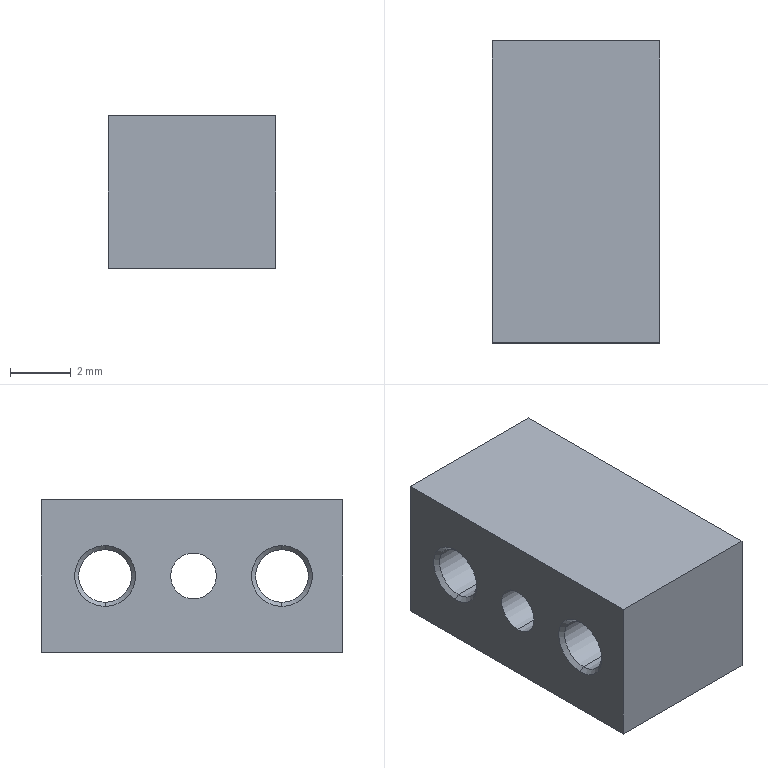Part | STEP file | 1 solid | 20 faces | box 5.5 x 9.9 x 5 mm | volume 236.494 mm3 | cone 8 | cylinder 6 | plane 6 | commonest cylinder face diameters 1.729 x4 1.5 x2
STEP:
#1=CARTESIAN_POINT('',(0.,0.,0.));
#2=DIRECTION('',(0.,0.,1.));
#3=DIRECTION('',(1.,0.,0.));
#4=AXIS2_PLACEMENT_3D('',#1,#2,#3);
#5=CARTESIAN_POINT('',(5.364,7.8,-0.8645));
#6=VERTEX_POINT('',#5);
#7=CARTESIAN_POINT('',(5.5,7.8,-1.));
#8=VERTEX_POINT('',#7);
#9=CARTESIAN_POINT('',(5.5,7.8,-1.));
#10=DIRECTION('',(0.7071,0.,-0.7071));
#11=VECTOR('',#10,1.);
#12=LINE('',#9,#11);
#13=CARTESIAN_POINT('',(5.5,7.8,0.));
#14=DIRECTION('',(1.,0.,0.));
#15=DIRECTION('',(0.,0.,-1.));
#16=AXIS2_PLACEMENT_3D('',#13,#14,#15);
#17=CONICAL_SURFACE('',#16,1.,0.7854);
#18=CARTESIAN_POINT('',(6.283,0.));
#19=DIRECTION('',(0.,1.));
#20=VECTOR('',#19,1.);
#21=LINE('',#18,#20);
#22=(GEOMETRIC_REPRESENTATION_CONTEXT(2)PARAMETRIC_REPRESENTATION_CONTEXT()REPRESENTATION_CONTEXT('',''));
#23=DEFINITIONAL_REPRESENTATION('',(#21),#22);
#24=PCURVE('',#17,#23);
#25=CARTESIAN_POINT('',(5.5,7.8,0.));
#26=DIRECTION('',(1.,0.,0.));
#27=DIRECTION('',(0.,0.,-1.));
#28=AXIS2_PLACEMENT_3D('',#25,#26,#27);
#29=CONICAL_SURFACE('',#28,1.,0.7854);
#30=CARTESIAN_POINT('',(0.,0.));
#31=DIRECTION('',(0.,1.));
#32=VECTOR('',#31,1.);
#33=LINE('',#30,#32);
#34=(GEOMETRIC_REPRESENTATION_CONTEXT(2)PARAMETRIC_REPRESENTATION_CONTEXT()REPRESENTATION_CONTEXT('',''));
#35=DEFINITIONAL_REPRESENTATION('',(#33),#34);
#36=PCURVE('',#29,#35);
#37=SURFACE_CURVE('',#12,(#24,#36),.PCURVE_S1.);
#38=EDGE_CURVE('',#6,#8,#37,.T.);
#39=ORIENTED_EDGE('',*,*,#38,.T.);
#40=CARTESIAN_POINT('',(5.5,7.8,1.));
#41=VERTEX_POINT('',#40);
#42=CARTESIAN_POINT('',(5.5,7.8,0.));
#43=DIRECTION('',(1.,0.,0.));
#44=DIRECTION('',(0.,0.,-1.));
#45=AXIS2_PLACEMENT_3D('',#42,#43,#44);
#46=CIRCLE('',#45,1.);
#47=CARTESIAN_POINT('',(0.,0.));
#48=DIRECTION('',(1.,0.));
#49=VECTOR('',#48,1.);
#50=LINE('',#47,#49);
#51=(GEOMETRIC_REPRESENTATION_CONTEXT(2)PARAMETRIC_REPRESENTATION_CONTEXT()REPRESENTATION_CONTEXT('',''));
#52=DEFINITIONAL_REPRESENTATION('',(#50),#51);
#53=PCURVE('',#17,#52);
#54=CARTESIAN_POINT('',(5.5,0.,2.5));
#55=DIRECTION('',(-1.,0.,0.));
#56=DIRECTION('',(0.,0.,1.));
#57=AXIS2_PLACEMENT_3D('',#54,#55,#56);
#58=PLANE('',#57);
#59=CARTESIAN_POINT('',(-3.5,7.8));
#60=CARTESIAN_POINT('',(-3.5,9.532));
#61=CARTESIAN_POINT('',(-2.,8.666));
#62=CARTESIAN_POINT('',(-0.5,7.8));
#63=CARTESIAN_POINT('',(-2.,6.934));
#64=CARTESIAN_POINT('',(-3.5,6.068));
#65=CARTESIAN_POINT('',(-3.5,7.8));
#66=(BOUNDED_CURVE()B_SPLINE_CURVE(2,(#59,#60,#61,#62,#63,#64,#65),.UNSPECIFIED.,.T.,.F.)B_SPLINE_CURVE_WITH_KNOTS((1,2,2,2,2,1),(-2.094,0.,2.094,4.189,6.283,8.378),.UNSPECIFIED.)CURVE()GEOMETRIC_REPRESENTATION_ITEM()RATIONAL_B_SPLINE_CURVE((1.,0.5,1.,0.5,1.,0.5,1.))REPRESENTATION_ITEM(''));
#67=(GEOMETRIC_REPRESENTATION_CONTEXT(2)PARAMETRIC_REPRESENTATION_CONTEXT()REPRESENTATION_CONTEXT('',''));
#68=DEFINITIONAL_REPRESENTATION('',(#66),#67);
#69=PCURVE('',#58,#68);
#70=SURFACE_CURVE('',#46,(#53,#69),.PCURVE_S1.);
#71=EDGE_CURVE('',#41,#8,#70,.T.);
#72=ORIENTED_EDGE('',*,*,#71,.F.);
#73=CARTESIAN_POINT('',(5.364,7.8,0.8645));
#74=VERTEX_POINT('',#73);
#75=CARTESIAN_POINT('',(5.5,7.8,1.));
#76=DIRECTION('',(0.7071,0.,0.7071));
#77=VECTOR('',#76,1.);
#78=LINE('',#75,#77);
#79=CARTESIAN_POINT('',(3.142,0.));
#80=DIRECTION('',(0.,1.));
#81=VECTOR('',#80,1.);
#82=LINE('',#79,#81);
#83=(GEOMETRIC_REPRESENTATION_CONTEXT(2)PARAMETRIC_REPRESENTATION_CONTEXT()REPRESENTATION_CONTEXT('',''));
#84=DEFINITIONAL_REPRESENTATION('',(#82),#83);
#85=PCURVE('',#17,#84);
#86=CARTESIAN_POINT('',(3.142,0.));
#87=DIRECTION('',(0.,1.));
#88=VECTOR('',#87,1.);
#89=LINE('',#86,#88);
#90=(GEOMETRIC_REPRESENTATION_CONTEXT(2)PARAMETRIC_REPRESENTATION_CONTEXT()REPRESENTATION_CONTEXT('',''));
#91=DEFINITIONAL_REPRESENTATION('',(#89),#90);
#92=PCURVE('',#29,#91);
#93=SURFACE_CURVE('',#78,(#85,#92),.PCURVE_S1.);
#94=EDGE_CURVE('',#74,#41,#93,.T.);
#95=ORIENTED_EDGE('',*,*,#94,.F.);
#96=CARTESIAN_POINT('',(5.364,7.8,0.));
#97=DIRECTION('',(1.,0.,0.));
#98=DIRECTION('',(0.,0.,-1.));
#99=AXIS2_PLACEMENT_3D('',#96,#97,#98);
#100=CIRCLE('',#99,0.8645);
#101=CARTESIAN_POINT('',(0.,-0.1355));
#102=DIRECTION('',(1.,0.));
#103=VECTOR('',#102,1.);
#104=LINE('',#101,#103);
#105=(GEOMETRIC_REPRESENTATION_CONTEXT(2)PARAMETRIC_REPRESENTATION_CONTEXT()REPRESENTATION_CONTEXT('',''));
#106=DEFINITIONAL_REPRESENTATION('',(#104),#105);
#107=PCURVE('',#17,#106);
#108=CARTESIAN_POINT('',(5.5,7.8,0.));
#109=DIRECTION('',(1.,0.,0.));
#110=DIRECTION('',(0.,0.,-1.));
#111=AXIS2_PLACEMENT_3D('',#108,#109,#110);
#112=CYLINDRICAL_SURFACE('',#111,0.8645);
#113=CARTESIAN_POINT('',(0.,-0.1355));
#114=DIRECTION('',(1.,0.));
#115=VECTOR('',#114,1.);
#116=LINE('',#113,#115);
#117=(GEOMETRIC_REPRESENTATION_CONTEXT(2)PARAMETRIC_REPRESENTATION_CONTEXT()REPRESENTATION_CONTEXT('',''));
#118=DEFINITIONAL_REPRESENTATION('',(#116),#117);
#119=PCURVE('',#112,#118);
#120=SURFACE_CURVE('',#100,(#107,#119),.PCURVE_S1.);
#121=EDGE_CURVE('',#74,#6,#120,.T.);
#122=ORIENTED_EDGE('',*,*,#121,.T.);
#123=EDGE_LOOP('',(#39,#72,#95,#122));
#124=FACE_BOUND('',#123,.F.);
#125=ADVANCED_FACE('',(#124),#17,.F.);
#126=CARTESIAN_POINT('',(0.1355,7.8,-0.8645));
#127=VERTEX_POINT('',#126);
#128=CARTESIAN_POINT('',(5.5,7.8,-0.8645));
#129=DIRECTION('',(1.,0.,0.));
#130=VECTOR('',#129,1.);
#131=LINE('',#128,#130);
#132=CARTESIAN_POINT('',(6.283,0.));
#133=DIRECTION('',(0.,1.));
#134=VECTOR('',#133,1.);
#135=LINE('',#132,#134);
#136=(GEOMETRIC_REPRESENTATION_CONTEXT(2)PARAMETRIC_REPRESENTATION_CONTEXT()REPRESENTATION_CONTEXT('',''));
#137=DEFINITIONAL_REPRESENTATION('',(#135),#136);
#138=PCURVE('',#112,#137);
#139=CARTESIAN_POINT('',(5.5,7.8,0.));
#140=DIRECTION('',(1.,0.,0.));
#141=DIRECTION('',(0.,0.,-1.));
#142=AXIS2_PLACEMENT_3D('',#139,#140,#141);
#143=CYLINDRICAL_SURFACE('',#142,0.8645);
#144=CARTESIAN_POINT('',(0.,0.));
#145=DIRECTION('',(0.,1.));
#146=VECTOR('',#145,1.);
#147=LINE('',#144,#146);
#148=(GEOMETRIC_REPRESENTATION_CONTEXT(2)PARAMETRIC_REPRESENTATION_CONTEXT()REPRESENTATION_CONTEXT('',''));
#149=DEFINITIONAL_REPRESENTATION('',(#147),#148);
#150=PCURVE('',#143,#149);
#151=SURFACE_CURVE('',#131,(#138,#150),.PCURVE_S1.);
#152=EDGE_CURVE('',#127,#6,#151,.T.);
#153=ORIENTED_EDGE('',*,*,#152,.T.);
#154=ORIENTED_EDGE('',*,*,#121,.F.);
#155=CARTESIAN_POINT('',(0.1355,7.8,0.8645));
#156=VERTEX_POINT('',#155);
#157=CARTESIAN_POINT('',(5.5,7.8,0.8645));
#158=DIRECTION('',(1.,0.,0.));
#159=VECTOR('',#158,1.);
#160=LINE('',#157,#159);
#161=CARTESIAN_POINT('',(3.142,0.));
#162=DIRECTION('',(0.,1.));
#163=VECTOR('',#162,1.);
#164=LINE('',#161,#163);
#165=(GEOMETRIC_REPRESENTATION_CONTEXT(2)PARAMETRIC_REPRESENTATION_CONTEXT()REPRESENTATION_CONTEXT('',''));
#166=DEFINITIONAL_REPRESENTATION('',(#164),#165);
#167=PCURVE('',#112,#166);
#168=CARTESIAN_POINT('',(3.142,0.));
#169=DIRECTION('',(0.,1.));
#170=VECTOR('',#169,1.);
#171=LINE('',#168,#170);
#172=(GEOMETRIC_REPRESENTATION_CONTEXT(2)PARAMETRIC_REPRESENTATION_CONTEXT()REPRESENTATION_CONTEXT('',''));
#173=DEFINITIONAL_REPRESENTATION('',(#171),#172);
#174=PCURVE('',#143,#173);
#175=SURFACE_CURVE('',#160,(#167,#174),.PCURVE_S1.);
#176=EDGE_CURVE('',#156,#74,#175,.T.);
#177=ORIENTED_EDGE('',*,*,#176,.F.);
#178=CARTESIAN_POINT('',(0.1355,7.8,0.));
#179=DIRECTION('',(1.,0.,0.));
#180=DIRECTION('',(0.,0.,-1.));
#181=AXIS2_PLACEMENT_3D('',#178,#179,#180);
#182=CIRCLE('',#181,0.8645);
#183=CARTESIAN_POINT('',(0.,-5.364));
#184=DIRECTION('',(1.,0.));
#185=VECTOR('',#184,1.);
#186=LINE('',#183,#185);
#187=(GEOMETRIC_REPRESENTATION_CONTEXT(2)PARAMETRIC_REPRESENTATION_CONTEXT()REPRESENTATION_CONTEXT('',''));
#188=DEFINITIONAL_REPRESENTATION('',(#186),#187);
#189=PCURVE('',#112,#188);
#190=CARTESIAN_POINT('',(0.1355,7.8,0.));
#191=DIRECTION('',(-1.,0.,0.));
#192=DIRECTION('',(0.,0.,1.));
#193=AXIS2_PLACEMENT_3D('',#190,#191,#192);
#194=CONICAL_SURFACE('',#193,0.8645,0.7854);
#195=CARTESIAN_POINT('',(9.425,0.));
#196=DIRECTION('',(-1.,0.));
#197=VECTOR('',#196,1.);
#198=LINE('',#195,#197);
#199=(GEOMETRIC_REPRESENTATION_CONTEXT(2)PARAMETRIC_REPRESENTATION_CONTEXT()REPRESENTATION_CONTEXT('',''));
#200=DEFINITIONAL_REPRESENTATION('',(#198),#199);
#201=PCURVE('',#194,#200);
#202=SURFACE_CURVE('',#182,(#189,#201),.PCURVE_S1.);
#203=EDGE_CURVE('',#156,#127,#202,.T.);
#204=ORIENTED_EDGE('',*,*,#203,.T.);
#205=EDGE_LOOP('',(#153,#154,#177,#204));
#206=FACE_BOUND('',#205,.F.);
#207=ADVANCED_FACE('',(#206),#112,.F.);
#208=CARTESIAN_POINT('',(0.,7.8,1.));
#209=VERTEX_POINT('',#208);
#210=CARTESIAN_POINT('',(0.1355,7.8,0.8645));
#211=DIRECTION('',(-0.7071,0.,0.7071));
#212=VECTOR('',#211,1.);
#213=LINE('',#210,#212);
#214=CARTESIAN_POINT('',(6.283,0.));
#215=DIRECTION('',(0.,1.));
#216=VECTOR('',#215,1.);
#217=LINE('',#214,#216);
#218=(GEOMETRIC_REPRESENTATION_CONTEXT(2)PARAMETRIC_REPRESENTATION_CONTEXT()REPRESENTATION_CONTEXT('',''));
#219=DEFINITIONAL_REPRESENTATION('',(#217),#218);
#220=PCURVE('',#194,#219);
#221=CARTESIAN_POINT('',(0.1355,7.8,0.));
#222=DIRECTION('',(-1.,0.,0.));
#223=DIRECTION('',(0.,0.,1.));
#224=AXIS2_PLACEMENT_3D('',#221,#222,#223);
#225=CONICAL_SURFACE('',#224,0.8645,0.7854);
#226=CARTESIAN_POINT('',(0.,0.));
#227=DIRECTION('',(0.,1.));
#228=VECTOR('',#227,1.);
#229=LINE('',#226,#228);
#230=(GEOMETRIC_REPRESENTATION_CONTEXT(2)PARAMETRIC_REPRESENTATION_CONTEXT()REPRESENTATION_CONTEXT('',''));
#231=DEFINITIONAL_REPRESENTATION('',(#229),#230);
#232=PCURVE('',#225,#231);
#233=SURFACE_CURVE('',#213,(#220,#232),.PCURVE_S1.);
#234=EDGE_CURVE('',#156,#209,#233,.T.);
#235=ORIENTED_EDGE('',*,*,#234,.T.);
#236=CARTESIAN_POINT('',(0.,7.8,-1.));
#237=VERTEX_POINT('',#236);
#238=CARTESIAN_POINT('',(0.,7.8,0.));
#239=DIRECTION('',(1.,0.,0.));
#240=DIRECTION('',(0.,0.,-1.));
#241=AXIS2_PLACEMENT_3D('',#238,#239,#240);
#242=CIRCLE('',#241,1.);
#243=CARTESIAN_POINT('',(9.425,0.1355));
#244=DIRECTION('',(-1.,0.));
#245=VECTOR('',#244,1.);
#246=LINE('',#243,#245);
#247=(GEOMETRIC_REPRESENTATION_CONTEXT(2)PARAMETRIC_REPRESENTATION_CONTEXT()REPRESENTATION_CONTEXT('',''));
#248=DEFINITIONAL_REPRESENTATION('',(#246),#247);
#249=PCURVE('',#194,#248);
#250=CARTESIAN_POINT('',(0.,9.9,2.5));
#251=DIRECTION('',(1.,0.,0.));
#252=DIRECTION('',(0.,0.,-1.));
#253=AXIS2_PLACEMENT_3D('',#250,#251,#252);
#254=PLANE('',#253);
#255=CARTESIAN_POINT('',(2.5,-2.1));
#256=DIRECTION('',(1.,0.));
#257=AXIS2_PLACEMENT_2D('',#255,#256);
#258=CIRCLE('',#257,1.);
#259=(GEOMETRIC_REPRESENTATION_CONTEXT(2)PARAMETRIC_REPRESENTATION_CONTEXT()REPRESENTATION_CONTEXT('',''));
#260=DEFINITIONAL_REPRESENTATION('',(#258),#259);
#261=PCURVE('',#254,#260);
#262=SURFACE_CURVE('',#242,(#249,#261),.PCURVE_S1.);
#263=EDGE_CURVE('',#209,#237,#262,.T.);
#264=ORIENTED_EDGE('',*,*,#263,.T.);
#265=CARTESIAN_POINT('',(0.1355,7.8,-0.8645));
#266=DIRECTION('',(-0.7071,0.,-0.7071));
#267=VECTOR('',#266,1.);
#268=LINE('',#265,#267);
#269=CARTESIAN_POINT('',(3.142,0.));
#270=DIRECTION('',(0.,1.));
#271=VECTOR('',#270,1.);
#272=LINE('',#269,#271);
#273=(GEOMETRIC_REPRESENTATION_CONTEXT(2)PARAMETRIC_REPRESENTATION_CONTEXT()REPRESENTATION_CONTEXT('',''));
#274=DEFINITIONAL_REPRESENTATION('',(#272),#273);
#275=PCURVE('',#194,#274);
#276=CARTESIAN_POINT('',(3.142,0.));
#277=DIRECTION('',(0.,1.));
#278=VECTOR('',#277,1.);
#279=LINE('',#276,#278);
#280=(GEOMETRIC_REPRESENTATION_CONTEXT(2)PARAMETRIC_REPRESENTATION_CONTEXT()REPRESENTATION_CONTEXT('',''));
#281=DEFINITIONAL_REPRESENTATION('',(#279),#280);
#282=PCURVE('',#225,#281);
#283=SURFACE_CURVE('',#268,(#275,#282),.PCURVE_S1.);
#284=EDGE_CURVE('',#127,#237,#283,.T.);
#285=ORIENTED_EDGE('',*,*,#284,.F.);
#286=ORIENTED_EDGE('',*,*,#203,.F.);
#287=EDGE_LOOP('',(#235,#264,#285,#286));
#288=FACE_BOUND('',#287,.F.);
#289=ADVANCED_FACE('',(#288),#194,.F.);
#290=CARTESIAN_POINT('',(5.364,2.,-0.8645));
#291=VERTEX_POINT('',#290);
#292=CARTESIAN_POINT('',(5.5,2.,-1.));
#293=VERTEX_POINT('',#292);
#294=CARTESIAN_POINT('',(5.5,2.,-1.));
#295=DIRECTION('',(0.7071,0.,-0.7071));
#296=VECTOR('',#295,1.);
#297=LINE('',#294,#296);
#298=CARTESIAN_POINT('',(5.5,2.,0.));
#299=DIRECTION('',(1.,0.,0.));
#300=DIRECTION('',(0.,0.,-1.));
#301=AXIS2_PLACEMENT_3D('',#298,#299,#300);
#302=CONICAL_SURFACE('',#301,1.,0.7854);
#303=CARTESIAN_POINT('',(6.283,0.));
#304=DIRECTION('',(0.,1.));
#305=VECTOR('',#304,1.);
#306=LINE('',#303,#305);
#307=(GEOMETRIC_REPRESENTATION_CONTEXT(2)PARAMETRIC_REPRESENTATION_CONTEXT()REPRESENTATION_CONTEXT('',''));
#308=DEFINITIONAL_REPRESENTATION('',(#306),#307);
#309=PCURVE('',#302,#308);
#310=CARTESIAN_POINT('',(5.5,2.,0.));
#311=DIRECTION('',(1.,0.,0.));
#312=DIRECTION('',(0.,0.,-1.));
#313=AXIS2_PLACEMENT_3D('',#310,#311,#312);
#314=CONICAL_SURFACE('',#313,1.,0.7854);
#315=CARTESIAN_POINT('',(0.,0.));
#316=DIRECTION('',(0.,1.));
#317=VECTOR('',#316,1.);
#318=LINE('',#315,#317);
#319=(GEOMETRIC_REPRESENTATION_CONTEXT(2)PARAMETRIC_REPRESENTATION_CONTEXT()REPRESENTATION_CONTEXT('',''));
#320=DEFINITIONAL_REPRESENTATION('',(#318),#319);
#321=PCURVE('',#314,#320);
#322=SURFACE_CURVE('',#297,(#309,#321),.PCURVE_S1.);
#323=EDGE_CURVE('',#291,#293,#322,.T.);
#324=ORIENTED_EDGE('',*,*,#323,.T.);
#325=CARTESIAN_POINT('',(5.5,2.,1.));
#326=VERTEX_POINT('',#325);
#327=CARTESIAN_POINT('',(5.5,2.,0.));
#328=DIRECTION('',(1.,0.,0.));
#329=DIRECTION('',(0.,0.,-1.));
#330=AXIS2_PLACEMENT_3D('',#327,#328,#329);
#331=CIRCLE('',#330,1.);
#332=CARTESIAN_POINT('',(0.,0.));
#333=DIRECTION('',(1.,0.));
#334=VECTOR('',#333,1.);
#335=LINE('',#332,#334);
#336=(GEOMETRIC_REPRESENTATION_CONTEXT(2)PARAMETRIC_REPRESENTATION_CONTEXT()REPRESENTATION_CONTEXT('',''));
#337=DEFINITIONAL_REPRESENTATION('',(#335),#336);
#338=PCURVE('',#302,#337);
#339=CARTESIAN_POINT('',(-3.5,2.));
#340=CARTESIAN_POINT('',(-3.5,3.732));
#341=CARTESIAN_POINT('',(-2.,2.866));
#342=CARTESIAN_POINT('',(-0.5,2.));
#343=CARTESIAN_POINT('',(-2.,1.134));
#344=CARTESIAN_POINT('',(-3.5,0.2679));
#345=CARTESIAN_POINT('',(-3.5,2.));
#346=(BOUNDED_CURVE()B_SPLINE_CURVE(2,(#339,#340,#341,#342,#343,#344,#345),.UNSPECIFIED.,.T.,.F.)B_SPLINE_CURVE_WITH_KNOTS((1,2,2,2,2,1),(-2.094,0.,2.094,4.189,6.283,8.378),.UNSPECIFIED.)CURVE()GEOMETRIC_REPRESENTATION_ITEM()RATIONAL_B_SPLINE_CURVE((1.,0.5,1.,0.5,1.,0.5,1.))REPRESENTATION_ITEM(''));
#347=(GEOMETRIC_REPRESENTATION_CONTEXT(2)PARAMETRIC_REPRESENTATION_CONTEXT()REPRESENTATION_CONTEXT('',''));
#348=DEFINITIONAL_REPRESENTATION('',(#346),#347);
#349=PCURVE('',#58,#348);
#350=SURFACE_CURVE('',#331,(#338,#349),.PCURVE_S1.);
#351=EDGE_CURVE('',#326,#293,#350,.T.);
#352=ORIENTED_EDGE('',*,*,#351,.F.);
#353=CARTESIAN_POINT('',(5.364,2.,0.8645));
#354=VERTEX_POINT('',#353);
#355=CARTESIAN_POINT('',(5.5,2.,1.));
#356=DIRECTION('',(0.7071,0.,0.7071));
#357=VECTOR('',#356,1.);
#358=LINE('',#355,#357);
#359=CARTESIAN_POINT('',(3.142,0.));
#360=DIRECTION('',(0.,1.));
#361=VECTOR('',#360,1.);
#362=LINE('',#359,#361);
#363=(GEOMETRIC_REPRESENTATION_CONTEXT(2)PARAMETRIC_REPRESENTATION_CONTEXT()REPRESENTATION_CONTEXT('',''));
#364=DEFINITIONAL_REPRESENTATION('',(#362),#363);
#365=PCURVE('',#302,#364);
#366=CARTESIAN_POINT('',(3.142,0.));
#367=DIRECTION('',(0.,1.));
#368=VECTOR('',#367,1.);
#369=LINE('',#366,#368);
#370=(GEOMETRIC_REPRESENTATION_CONTEXT(2)PARAMETRIC_REPRESENTATION_CONTEXT()REPRESENTATION_CONTEXT('',''));
#371=DEFINITIONAL_REPRESENTATION('',(#369),#370);
#372=PCURVE('',#314,#371);
#373=SURFACE_CURVE('',#358,(#365,#372),.PCURVE_S1.);
#374=EDGE_CURVE('',#354,#326,#373,.T.);
#375=ORIENTED_EDGE('',*,*,#374,.F.);
#376=CARTESIAN_POINT('',(5.364,2.,0.));
#377=DIRECTION('',(1.,0.,0.));
#378=DIRECTION('',(0.,0.,-1.));
#379=AXIS2_PLACEMENT_3D('',#376,#377,#378);
#380=CIRCLE('',#379,0.8645);
#381=CARTESIAN_POINT('',(0.,-0.1355));
#382=DIRECTION('',(1.,0.));
#383=VECTOR('',#382,1.);
#384=LINE('',#381,#383);
#385=(GEOMETRIC_REPRESENTATION_CONTEXT(2)PARAMETRIC_REPRESENTATION_CONTEXT()REPRESENTATION_CONTEXT('',''));
#386=DEFINITIONAL_REPRESENTATION('',(#384),#385);
#387=PCURVE('',#302,#386);
#388=CARTESIAN_POINT('',(5.5,2.,0.));
#389=DIRECTION('',(1.,0.,0.));
#390=DIRECTION('',(0.,0.,-1.));
#391=AXIS2_PLACEMENT_3D('',#388,#389,#390);
#392=CYLINDRICAL_SURFACE('',#391,0.8645);
#393=CARTESIAN_POINT('',(0.,-0.1355));
#394=DIRECTION('',(1.,0.));
#395=VECTOR('',#394,1.);
#396=LINE('',#393,#395);
#397=(GEOMETRIC_REPRESENTATION_CONTEXT(2)PARAMETRIC_REPRESENTATION_CONTEXT()REPRESENTATION_CONTEXT('',''));
#398=DEFINITIONAL_REPRESENTATION('',(#396),#397);
#399=PCURVE('',#392,#398);
#400=SURFACE_CURVE('',#380,(#387,#399),.PCURVE_S1.);
#401=EDGE_CURVE('',#354,#291,#400,.T.);
#402=ORIENTED_EDGE('',*,*,#401,.T.);
#403=EDGE_LOOP('',(#324,#352,#375,#402));
#404=FACE_BOUND('',#403,.F.);
#405=ADVANCED_FACE('',(#404),#302,.F.);
#406=CARTESIAN_POINT('',(0.1355,2.,-0.8645));
#407=VERTEX_POINT('',#406);
#408=CARTESIAN_POINT('',(5.5,2.,-0.8645));
#409=DIRECTION('',(1.,0.,0.));
#410=VECTOR('',#409,1.);
#411=LINE('',#408,#410);
#412=CARTESIAN_POINT('',(6.283,0.));
#413=DIRECTION('',(0.,1.));
#414=VECTOR('',#413,1.);
#415=LINE('',#412,#414);
#416=(GEOMETRIC_REPRESENTATION_CONTEXT(2)PARAMETRIC_REPRESENTATION_CONTEXT()REPRESENTATION_CONTEXT('',''));
#417=DEFINITIONAL_REPRESENTATION('',(#415),#416);
#418=PCURVE('',#392,#417);
#419=CARTESIAN_POINT('',(5.5,2.,0.));
#420=DIRECTION('',(1.,0.,0.));
#421=DIRECTION('',(0.,0.,-1.));
#422=AXIS2_PLACEMENT_3D('',#419,#420,#421);
#423=CYLINDRICAL_SURFACE('',#422,0.8645);
#424=CARTESIAN_POINT('',(0.,0.));
#425=DIRECTION('',(0.,1.));
#426=VECTOR('',#425,1.);
#427=LINE('',#424,#426);
#428=(GEOMETRIC_REPRESENTATION_CONTEXT(2)PARAMETRIC_REPRESENTATION_CONTEXT()REPRESENTATION_CONTEXT('',''));
#429=DEFINITIONAL_REPRESENTATION('',(#427),#428);
#430=PCURVE('',#423,#429);
#431=SURFACE_CURVE('',#411,(#418,#430),.PCURVE_S1.);
#432=EDGE_CURVE('',#407,#291,#431,.T.);
#433=ORIENTED_EDGE('',*,*,#432,.T.);
#434=ORIENTED_EDGE('',*,*,#401,.F.);
#435=CARTESIAN_POINT('',(0.1355,2.,0.8645));
#436=VERTEX_POINT('',#435);
#437=CARTESIAN_POINT('',(5.5,2.,0.8645));
#438=DIRECTION('',(1.,0.,0.));
#439=VECTOR('',#438,1.);
#440=LINE('',#437,#439);
#441=CARTESIAN_POINT('',(3.142,0.));
#442=DIRECTION('',(0.,1.));
#443=VECTOR('',#442,1.);
#444=LINE('',#441,#443);
#445=(GEOMETRIC_REPRESENTATION_CONTEXT(2)PARAMETRIC_REPRESENTATION_CONTEXT()REPRESENTATION_CONTEXT('',''));
#446=DEFINITIONAL_REPRESENTATION('',(#444),#445);
#447=PCURVE('',#392,#446);
#448=CARTESIAN_POINT('',(3.142,0.));
#449=DIRECTION('',(0.,1.));
#450=VECTOR('',#449,1.);
#451=LINE('',#448,#450);
#452=(GEOMETRIC_REPRESENTATION_CONTEXT(2)PARAMETRIC_REPRESENTATION_CONTEXT()REPRESENTATION_CONTEXT('',''));
#453=DEFINITIONAL_REPRESENTATION('',(#451),#452);
#454=PCURVE('',#423,#453);
#455=SURFACE_CURVE('',#440,(#447,#454),.PCURVE_S1.);
#456=EDGE_CURVE('',#436,#354,#455,.T.);
#457=ORIENTED_EDGE('',*,*,#456,.F.);
#458=CARTESIAN_POINT('',(0.1355,2.,0.));
#459=DIRECTION('',(1.,0.,0.));
#460=DIRECTION('',(0.,0.,-1.));
#461=AXIS2_PLACEMENT_3D('',#458,#459,#460);
#462=CIRCLE('',#461,0.8645);
#463=CARTESIAN_POINT('',(0.,-5.364));
#464=DIRECTION('',(1.,0.));
#465=VECTOR('',#464,1.);
#466=LINE('',#463,#465);
#467=(GEOMETRIC_REPRESENTATION_CONTEXT(2)PARAMETRIC_REPRESENTATION_CONTEXT()REPRESENTATION_CONTEXT('',''));
#468=DEFINITIONAL_REPRESENTATION('',(#466),#467);
#469=PCURVE('',#392,#468);
#470=CARTESIAN_POINT('',(0.1355,2.,0.));
#471=DIRECTION('',(-1.,0.,0.));
#472=DIRECTION('',(0.,0.,1.));
#473=AXIS2_PLACEMENT_3D('',#470,#471,#472);
#474=CONICAL_SURFACE('',#473,0.8645,0.7854);
#475=CARTESIAN_POINT('',(9.425,0.));
#476=DIRECTION('',(-1.,0.));
#477=VECTOR('',#476,1.);
#478=LINE('',#475,#477);
#479=(GEOMETRIC_REPRESENTATION_CONTEXT(2)PARAMETRIC_REPRESENTATION_CONTEXT()REPRESENTATION_CONTEXT('',''));
#480=DEFINITIONAL_REPRESENTATION('',(#478),#479);
#481=PCURVE('',#474,#480);
#482=SURFACE_CURVE('',#462,(#469,#481),.PCURVE_S1.);
#483=EDGE_CURVE('',#436,#407,#482,.T.);
#484=ORIENTED_EDGE('',*,*,#483,.T.);
#485=EDGE_LOOP('',(#433,#434,#457,#484));
#486=FACE_BOUND('',#485,.F.);
#487=ADVANCED_FACE('',(#486),#392,.F.);
#488=CARTESIAN_POINT('',(0.,2.,1.));
#489=VERTEX_POINT('',#488);
#490=CARTESIAN_POINT('',(0.1355,2.,0.8645));
#491=DIRECTION('',(-0.7071,0.,0.7071));
#492=VECTOR('',#491,1.);
#493=LINE('',#490,#492);
#494=CARTESIAN_POINT('',(6.283,0.));
#495=DIRECTION('',(0.,1.));
#496=VECTOR('',#495,1.);
#497=LINE('',#494,#496);
#498=(GEOMETRIC_REPRESENTATION_CONTEXT(2)PARAMETRIC_REPRESENTATION_CONTEXT()REPRESENTATION_CONTEXT('',''));
#499=DEFINITIONAL_REPRESENTATION('',(#497),#498);
#500=PCURVE('',#474,#499);
#501=CARTESIAN_POINT('',(0.1355,2.,0.));
#502=DIRECTION('',(-1.,0.,0.));
#503=DIRECTION('',(0.,0.,1.));
#504=AXIS2_PLACEMENT_3D('',#501,#502,#503);
#505=CONICAL_SURFACE('',#504,0.8645,0.7854);
#506=CARTESIAN_POINT('',(0.,0.));
#507=DIRECTION('',(0.,1.));
#508=VECTOR('',#507,1.);
#509=LINE('',#506,#508);
#510=(GEOMETRIC_REPRESENTATION_CONTEXT(2)PARAMETRIC_REPRESENTATION_CONTEXT()REPRESENTATION_CONTEXT('',''));
#511=DEFINITIONAL_REPRESENTATION('',(#509),#510);
#512=PCURVE('',#505,#511);
#513=SURFACE_CURVE('',#493,(#500,#512),.PCURVE_S1.);
#514=EDGE_CURVE('',#436,#489,#513,.T.);
#515=ORIENTED_EDGE('',*,*,#514,.T.);
#516=CARTESIAN_POINT('',(0.,2.,-1.));
#517=VERTEX_POINT('',#516);
#518=CARTESIAN_POINT('',(0.,2.,0.));
#519=DIRECTION('',(1.,0.,0.));
#520=DIRECTION('',(0.,0.,-1.));
#521=AXIS2_PLACEMENT_3D('',#518,#519,#520);
#522=CIRCLE('',#521,1.);
#523=CARTESIAN_POINT('',(9.425,0.1355));
#524=DIRECTION('',(-1.,0.));
#525=VECTOR('',#524,1.);
#526=LINE('',#523,#525);
#527=(GEOMETRIC_REPRESENTATION_CONTEXT(2)PARAMETRIC_REPRESENTATION_CONTEXT()REPRESENTATION_CONTEXT('',''));
#528=DEFINITIONAL_REPRESENTATION('',(#526),#527);
#529=PCURVE('',#474,#528);
#530=CARTESIAN_POINT('',(2.5,-7.9));
#531=DIRECTION('',(1.,0.));
#532=AXIS2_PLACEMENT_2D('',#530,#531);
#533=CIRCLE('',#532,1.);
#534=(GEOMETRIC_REPRESENTATION_CONTEXT(2)PARAMETRIC_REPRESENTATION_CONTEXT()REPRESENTATION_CONTEXT('',''));
#535=DEFINITIONAL_REPRESENTATION('',(#533),#534);
#536=PCURVE('',#254,#535);
#537=SURFACE_CURVE('',#522,(#529,#536),.PCURVE_S1.);
#538=EDGE_CURVE('',#489,#517,#537,.T.);
#539=ORIENTED_EDGE('',*,*,#538,.T.);
#540=CARTESIAN_POINT('',(0.1355,2.,-0.8645));
#541=DIRECTION('',(-0.7071,0.,-0.7071));
#542=VECTOR('',#541,1.);
#543=LINE('',#540,#542);
#544=CARTESIAN_POINT('',(3.142,0.));
#545=DIRECTION('',(0.,1.));
#546=VECTOR('',#545,1.);
#547=LINE('',#544,#546);
#548=(GEOMETRIC_REPRESENTATION_CONTEXT(2)PARAMETRIC_REPRESENTATION_CONTEXT()REPRESENTATION_CONTEXT('',''));
#549=DEFINITIONAL_REPRESENTATION('',(#547),#548);
#550=PCURVE('',#474,#549);
#551=CARTESIAN_POINT('',(3.142,0.));
#552=DIRECTION('',(0.,1.));
#553=VECTOR('',#552,1.);
#554=LINE('',#551,#553);
#555=(GEOMETRIC_REPRESENTATION_CONTEXT(2)PARAMETRIC_REPRESENTATION_CONTEXT()REPRESENTATION_CONTEXT('',''));
#556=DEFINITIONAL_REPRESENTATION('',(#554),#555);
#557=PCURVE('',#505,#556);
#558=SURFACE_CURVE('',#543,(#550,#557),.PCURVE_S1.);
#559=EDGE_CURVE('',#407,#517,#558,.T.);
#560=ORIENTED_EDGE('',*,*,#559,.F.);
#561=ORIENTED_EDGE('',*,*,#483,.F.);
#562=EDGE_LOOP('',(#515,#539,#560,#561));
#563=FACE_BOUND('',#562,.F.);
#564=ADVANCED_FACE('',(#563),#474,.F.);
#565=CARTESIAN_POINT('',(5.5,4.9,0.75));
#566=VERTEX_POINT('',#565);
#567=CARTESIAN_POINT('',(0.,4.9,0.75));
#568=VERTEX_POINT('',#567);
#569=CARTESIAN_POINT('',(0.,4.9,0.75));
#570=DIRECTION('',(-1.,0.,0.));
#571=VECTOR('',#570,1.);
#572=LINE('',#569,#571);
#573=CARTESIAN_POINT('',(0.,4.9,0.));
#574=DIRECTION('',(-1.,0.,0.));
#575=DIRECTION('',(0.,0.,1.));
#576=AXIS2_PLACEMENT_3D('',#573,#574,#575);
#577=CYLINDRICAL_SURFACE('',#576,0.75);
#578=CARTESIAN_POINT('',(6.283,0.));
#579=DIRECTION('',(0.,1.));
#580=VECTOR('',#579,1.);
#581=LINE('',#578,#580);
#582=(GEOMETRIC_REPRESENTATION_CONTEXT(2)PARAMETRIC_REPRESENTATION_CONTEXT()REPRESENTATION_CONTEXT('',''));
#583=DEFINITIONAL_REPRESENTATION('',(#581),#582);
#584=PCURVE('',#577,#583);
#585=CARTESIAN_POINT('',(0.,4.9,0.));
#586=DIRECTION('',(-1.,0.,0.));
#587=DIRECTION('',(0.,0.,1.));
#588=AXIS2_PLACEMENT_3D('',#585,#586,#587);
#589=CYLINDRICAL_SURFACE('',#588,0.75);
#590=CARTESIAN_POINT('',(0.,0.));
#591=DIRECTION('',(0.,1.));
#592=VECTOR('',#591,1.);
#593=LINE('',#590,#592);
#594=(GEOMETRIC_REPRESENTATION_CONTEXT(2)PARAMETRIC_REPRESENTATION_CONTEXT()REPRESENTATION_CONTEXT('',''));
#595=DEFINITIONAL_REPRESENTATION('',(#593),#594);
#596=PCURVE('',#589,#595);
#597=SURFACE_CURVE('',#572,(#584,#596),.PCURVE_S1.);
#598=EDGE_CURVE('',#566,#568,#597,.T.);
#599=ORIENTED_EDGE('',*,*,#598,.T.);
#600=CARTESIAN_POINT('',(0.,4.9,-0.75));
#601=VERTEX_POINT('',#600);
#602=CARTESIAN_POINT('',(0.,4.9,0.));
#603=DIRECTION('',(-1.,0.,0.));
#604=DIRECTION('',(0.,0.,1.));
#605=AXIS2_PLACEMENT_3D('',#602,#603,#604);
#606=CIRCLE('',#605,0.75);
#607=CARTESIAN_POINT('',(0.,0.));
#608=DIRECTION('',(1.,0.));
#609=VECTOR('',#608,1.);
#610=LINE('',#607,#609);
#611=(GEOMETRIC_REPRESENTATION_CONTEXT(2)PARAMETRIC_REPRESENTATION_CONTEXT()REPRESENTATION_CONTEXT('',''));
#612=DEFINITIONAL_REPRESENTATION('',(#610),#611);
#613=PCURVE('',#577,#612);
#614=CARTESIAN_POINT('',(1.75,-5.));
#615=CARTESIAN_POINT('',(1.75,-3.701));
#616=CARTESIAN_POINT('',(2.875,-4.35));
#617=CARTESIAN_POINT('',(4.,-5.));
#618=CARTESIAN_POINT('',(2.875,-5.65));
#619=CARTESIAN_POINT('',(1.75,-6.299));
#620=CARTESIAN_POINT('',(1.75,-5.));
#621=(BOUNDED_CURVE()B_SPLINE_CURVE(2,(#614,#615,#616,#617,#618,#619,#620),.UNSPECIFIED.,.T.,.F.)B_SPLINE_CURVE_WITH_KNOTS((1,2,2,2,2,1),(-2.094,0.,2.094,4.189,6.283,8.378),.UNSPECIFIED.)CURVE()GEOMETRIC_REPRESENTATION_ITEM()RATIONAL_B_SPLINE_CURVE((1.,0.5,1.,0.5,1.,0.5,1.))REPRESENTATION_ITEM(''));
#622=(GEOMETRIC_REPRESENTATION_CONTEXT(2)PARAMETRIC_REPRESENTATION_CONTEXT()REPRESENTATION_CONTEXT('',''));
#623=DEFINITIONAL_REPRESENTATION('',(#621),#622);
#624=PCURVE('',#254,#623);
#625=SURFACE_CURVE('',#606,(#613,#624),.PCURVE_S1.);
#626=EDGE_CURVE('',#601,#568,#625,.T.);
#627=ORIENTED_EDGE('',*,*,#626,.F.);
#628=CARTESIAN_POINT('',(5.5,4.9,-0.75));
#629=VERTEX_POINT('',#628);
#630=CARTESIAN_POINT('',(0.,4.9,-0.75));
#631=DIRECTION('',(-1.,0.,0.));
#632=VECTOR('',#631,1.);
#633=LINE('',#630,#632);
#634=CARTESIAN_POINT('',(3.142,0.));
#635=DIRECTION('',(0.,1.));
#636=VECTOR('',#635,1.);
#637=LINE('',#634,#636);
#638=(GEOMETRIC_REPRESENTATION_CONTEXT(2)PARAMETRIC_REPRESENTATION_CONTEXT()REPRESENTATION_CONTEXT('',''));
#639=DEFINITIONAL_REPRESENTATION('',(#637),#638);
#640=PCURVE('',#577,#639);
#641=CARTESIAN_POINT('',(3.142,0.));
#642=DIRECTION('',(0.,1.));
#643=VECTOR('',#642,1.);
#644=LINE('',#641,#643);
#645=(GEOMETRIC_REPRESENTATION_CONTEXT(2)PARAMETRIC_REPRESENTATION_CONTEXT()REPRESENTATION_CONTEXT('',''));
#646=DEFINITIONAL_REPRESENTATION('',(#644),#645);
#647=PCURVE('',#589,#646);
#648=SURFACE_CURVE('',#633,(#640,#647),.PCURVE_S1.);
#649=EDGE_CURVE('',#629,#601,#648,.T.);
#650=ORIENTED_EDGE('',*,*,#649,.F.);
#651=CARTESIAN_POINT('',(5.5,4.9,0.));
#652=DIRECTION('',(-1.,0.,0.));
#653=DIRECTION('',(0.,0.,1.));
#654=AXIS2_PLACEMENT_3D('',#651,#652,#653);
#655=CIRCLE('',#654,0.75);
#656=CARTESIAN_POINT('',(0.,-5.5));
#657=DIRECTION('',(1.,0.));
#658=VECTOR('',#657,1.);
#659=LINE('',#656,#658);
#660=(GEOMETRIC_REPRESENTATION_CONTEXT(2)PARAMETRIC_REPRESENTATION_CONTEXT()REPRESENTATION_CONTEXT('',''));
#661=DEFINITIONAL_REPRESENTATION('',(#659),#660);
#662=PCURVE('',#577,#661);
#663=CARTESIAN_POINT('',(-2.5,4.9));
#664=DIRECTION('',(1.,0.));
#665=AXIS2_PLACEMENT_2D('',#663,#664);
#666=CIRCLE('',#665,0.75);
#667=(GEOMETRIC_REPRESENTATION_CONTEXT(2)PARAMETRIC_REPRESENTATION_CONTEXT()REPRESENTATION_CONTEXT('',''));
#668=DEFINITIONAL_REPRESENTATION('',(#666),#667);
#669=PCURVE('',#58,#668);
#670=SURFACE_CURVE('',#655,(#662,#669),.PCURVE_S1.);
#671=EDGE_CURVE('',#629,#566,#670,.T.);
#672=ORIENTED_EDGE('',*,*,#671,.T.);
#673=EDGE_LOOP('',(#599,#627,#650,#672));
#674=FACE_BOUND('',#673,.F.);
#675=ADVANCED_FACE('',(#674),#577,.F.);
#676=CARTESIAN_POINT('',(5.5,9.9,2.5));
#677=VERTEX_POINT('',#676);
#678=CARTESIAN_POINT('',(5.5,9.9,-2.5));
#679=VERTEX_POINT('',#678);
#680=CARTESIAN_POINT('',(5.5,9.9,2.5));
#681=DIRECTION('',(0.,0.,-1.));
#682=VECTOR('',#681,1.);
#683=LINE('',#680,#682);
#684=CARTESIAN_POINT('',(5.5,9.9,2.5));
#685=DIRECTION('',(0.,-1.,0.));
#686=DIRECTION('',(0.,0.,-1.));
#687=AXIS2_PLACEMENT_3D('',#684,#685,#686);
#688=PLANE('',#687);
#689=CARTESIAN_POINT('',(0.,0.));
#690=DIRECTION('',(1.,0.));
#691=VECTOR('',#690,1.);
#692=LINE('',#689,#691);
#693=(GEOMETRIC_REPRESENTATION_CONTEXT(2)PARAMETRIC_REPRESENTATION_CONTEXT()REPRESENTATION_CONTEXT('',''));
#694=DEFINITIONAL_REPRESENTATION('',(#692),#693);
#695=PCURVE('',#688,#694);
#696=CARTESIAN_POINT('',(0.,9.9));
#697=DIRECTION('',(-1.,0.));
#698=VECTOR('',#697,1.);
#699=LINE('',#696,#698);
#700=(GEOMETRIC_REPRESENTATION_CONTEXT(2)PARAMETRIC_REPRESENTATION_CONTEXT()REPRESENTATION_CONTEXT('',''));
#701=DEFINITIONAL_REPRESENTATION('',(#699),#700);
#702=PCURVE('',#58,#701);
#703=SURFACE_CURVE('',#683,(#695,#702),.PCURVE_S1.);
#704=EDGE_CURVE('',#677,#679,#703,.T.);
#705=ORIENTED_EDGE('',*,*,#704,.T.);
#706=CARTESIAN_POINT('',(0.,9.9,-2.5));
#707=VERTEX_POINT('',#706);
#708=CARTESIAN_POINT('',(5.5,9.9,-2.5));
#709=DIRECTION('',(-1.,0.,0.));
#710=VECTOR('',#709,1.);
#711=LINE('',#708,#710);
#712=CARTESIAN_POINT('',(5.,0.));
#713=DIRECTION('',(0.,-1.));
#714=VECTOR('',#713,1.);
#715=LINE('',#712,#714);
#716=(GEOMETRIC_REPRESENTATION_CONTEXT(2)PARAMETRIC_REPRESENTATION_CONTEXT()REPRESENTATION_CONTEXT('',''));
#717=DEFINITIONAL_REPRESENTATION('',(#715),#716);
#718=PCURVE('',#688,#717);
#719=CARTESIAN_POINT('',(0.,9.9,-2.5));
#720=DIRECTION('',(0.,0.,1.));
#721=DIRECTION('',(1.,0.,0.));
#722=AXIS2_PLACEMENT_3D('',#719,#720,#721);
#723=PLANE('',#722);
#724=CARTESIAN_POINT('',(5.5,0.));
#725=DIRECTION('',(-1.,0.));
#726=VECTOR('',#725,1.);
#727=LINE('',#724,#726);
#728=(GEOMETRIC_REPRESENTATION_CONTEXT(2)PARAMETRIC_REPRESENTATION_CONTEXT()REPRESENTATION_CONTEXT('',''));
#729=DEFINITIONAL_REPRESENTATION('',(#727),#728);
#730=PCURVE('',#723,#729);
#731=SURFACE_CURVE('',#711,(#718,#730),.PCURVE_S1.);
#732=EDGE_CURVE('',#679,#707,#731,.T.);
#733=ORIENTED_EDGE('',*,*,#732,.T.);
#734=CARTESIAN_POINT('',(0.,9.9,2.5));
#735=VERTEX_POINT('',#734);
#736=CARTESIAN_POINT('',(0.,9.9,2.5));
#737=DIRECTION('',(0.,0.,-1.));
#738=VECTOR('',#737,1.);
#739=LINE('',#736,#738);
#740=CARTESIAN_POINT('',(0.,-5.5));
#741=DIRECTION('',(1.,0.));
#742=VECTOR('',#741,1.);
#743=LINE('',#740,#742);
#744=(GEOMETRIC_REPRESENTATION_CONTEXT(2)PARAMETRIC_REPRESENTATION_CONTEXT()REPRESENTATION_CONTEXT('',''));
#745=DEFINITIONAL_REPRESENTATION('',(#743),#744);
#746=PCURVE('',#688,#745);
#747=CARTESIAN_POINT('',(0.,0.));
#748=DIRECTION('',(1.,0.));
#749=VECTOR('',#748,1.);
#750=LINE('',#747,#749);
#751=(GEOMETRIC_REPRESENTATION_CONTEXT(2)PARAMETRIC_REPRESENTATION_CONTEXT()REPRESENTATION_CONTEXT('',''));
#752=DEFINITIONAL_REPRESENTATION('',(#750),#751);
#753=PCURVE('',#254,#752);
#754=SURFACE_CURVE('',#739,(#746,#753),.PCURVE_S1.);
#755=EDGE_CURVE('',#735,#707,#754,.T.);
#756=ORIENTED_EDGE('',*,*,#755,.F.);
#757=CARTESIAN_POINT('',(5.5,9.9,2.5));
#758=DIRECTION('',(-1.,0.,0.));
#759=VECTOR('',#758,1.);
#760=LINE('',#757,#759);
#761=CARTESIAN_POINT('',(0.,0.));
#762=DIRECTION('',(0.,-1.));
#763=VECTOR('',#762,1.);
#764=LINE('',#761,#763);
#765=(GEOMETRIC_REPRESENTATION_CONTEXT(2)PARAMETRIC_REPRESENTATION_CONTEXT()REPRESENTATION_CONTEXT('',''));
#766=DEFINITIONAL_REPRESENTATION('',(#764),#765);
#767=PCURVE('',#688,#766);
#768=CARTESIAN_POINT('',(0.,9.9,2.5));
#769=DIRECTION('',(0.,0.,1.));
#770=DIRECTION('',(1.,0.,0.));
#771=AXIS2_PLACEMENT_3D('',#768,#769,#770);
#772=PLANE('',#771);
#773=CARTESIAN_POINT('',(5.5,0.));
#774=DIRECTION('',(-1.,0.));
#775=VECTOR('',#774,1.);
#776=LINE('',#773,#775);
#777=(GEOMETRIC_REPRESENTATION_CONTEXT(2)PARAMETRIC_REPRESENTATION_CONTEXT()REPRESENTATION_CONTEXT('',''));
#778=DEFINITIONAL_REPRESENTATION('',(#776),#777);
#779=PCURVE('',#772,#778);
#780=SURFACE_CURVE('',#760,(#767,#779),.PCURVE_S1.);
#781=EDGE_CURVE('',#677,#735,#780,.T.);
#782=ORIENTED_EDGE('',*,*,#781,.F.);
#783=EDGE_LOOP('',(#705,#733,#756,#782));
#784=FACE_BOUND('',#783,.T.);
#785=ADVANCED_FACE('',(#784),#688,.F.);
#786=ORIENTED_EDGE('',*,*,#263,.T.);
#787=CARTESIAN_POINT('',(0.,7.8,0.));
#788=DIRECTION('',(1.,0.,0.));
#789=DIRECTION('',(0.,0.,-1.));
#790=AXIS2_PLACEMENT_3D('',#787,#788,#789);
#791=CIRCLE('',#790,1.);
#792=CARTESIAN_POINT('',(2.5,-2.1));
#793=DIRECTION('',(1.,0.));
#794=AXIS2_PLACEMENT_2D('',#792,#793);
#795=CIRCLE('',#794,1.);
#796=(GEOMETRIC_REPRESENTATION_CONTEXT(2)PARAMETRIC_REPRESENTATION_CONTEXT()REPRESENTATION_CONTEXT('',''));
#797=DEFINITIONAL_REPRESENTATION('',(#795),#796);
#798=PCURVE('',#254,#797);
#799=CARTESIAN_POINT('',(3.142,0.1355));
#800=DIRECTION('',(-1.,0.));
#801=VECTOR('',#800,1.);
#802=LINE('',#799,#801);
#803=(GEOMETRIC_REPRESENTATION_CONTEXT(2)PARAMETRIC_REPRESENTATION_CONTEXT()REPRESENTATION_CONTEXT('',''));
#804=DEFINITIONAL_REPRESENTATION('',(#802),#803);
#805=PCURVE('',#225,#804);
#806=SURFACE_CURVE('',#791,(#798,#805),.PCURVE_S1.);
#807=EDGE_CURVE('',#237,#209,#806,.T.);
#808=ORIENTED_EDGE('',*,*,#807,.T.);
#809=EDGE_LOOP('',(#786,#808));
#810=FACE_BOUND('',#809,.T.);
#811=ORIENTED_EDGE('',*,*,#538,.T.);
#812=CARTESIAN_POINT('',(0.,2.,0.));
#813=DIRECTION('',(1.,0.,0.));
#814=DIRECTION('',(0.,0.,-1.));
#815=AXIS2_PLACEMENT_3D('',#812,#813,#814);
#816=CIRCLE('',#815,1.);
#817=CARTESIAN_POINT('',(2.5,-7.9));
#818=DIRECTION('',(1.,0.));
#819=AXIS2_PLACEMENT_2D('',#817,#818);
#820=CIRCLE('',#819,1.);
#821=(GEOMETRIC_REPRESENTATION_CONTEXT(2)PARAMETRIC_REPRESENTATION_CONTEXT()REPRESENTATION_CONTEXT('',''));
#822=DEFINITIONAL_REPRESENTATION('',(#820),#821);
#823=PCURVE('',#254,#822);
#824=CARTESIAN_POINT('',(3.142,0.1355));
#825=DIRECTION('',(-1.,0.));
#826=VECTOR('',#825,1.);
#827=LINE('',#824,#826);
#828=(GEOMETRIC_REPRESENTATION_CONTEXT(2)PARAMETRIC_REPRESENTATION_CONTEXT()REPRESENTATION_CONTEXT('',''));
#829=DEFINITIONAL_REPRESENTATION('',(#827),#828);
#830=PCURVE('',#505,#829);
#831=SURFACE_CURVE('',#816,(#823,#830),.PCURVE_S1.);
#832=EDGE_CURVE('',#517,#489,#831,.T.);
#833=ORIENTED_EDGE('',*,*,#832,.T.);
#834=EDGE_LOOP('',(#811,#833));
#835=FACE_BOUND('',#834,.T.);
#836=CARTESIAN_POINT('',(0.,4.9,0.));
#837=DIRECTION('',(-1.,0.,0.));
#838=DIRECTION('',(0.,0.,1.));
#839=AXIS2_PLACEMENT_3D('',#836,#837,#838);
#840=CIRCLE('',#839,0.75);
#841=CARTESIAN_POINT('',(1.75,-5.));
#842=CARTESIAN_POINT('',(1.75,-3.701));
#843=CARTESIAN_POINT('',(2.875,-4.35));
#844=CARTESIAN_POINT('',(4.,-5.));
#845=CARTESIAN_POINT('',(2.875,-5.65));
#846=CARTESIAN_POINT('',(1.75,-6.299));
#847=CARTESIAN_POINT('',(1.75,-5.));
#848=(BOUNDED_CURVE()B_SPLINE_CURVE(2,(#841,#842,#843,#844,#845,#846,#847),.UNSPECIFIED.,.T.,.F.)B_SPLINE_CURVE_WITH_KNOTS((1,2,2,2,2,1),(-2.094,0.,2.094,4.189,6.283,8.378),.UNSPECIFIED.)CURVE()GEOMETRIC_REPRESENTATION_ITEM()RATIONAL_B_SPLINE_CURVE((1.,0.5,1.,0.5,1.,0.5,1.))REPRESENTATION_ITEM(''));
#849=(GEOMETRIC_REPRESENTATION_CONTEXT(2)PARAMETRIC_REPRESENTATION_CONTEXT()REPRESENTATION_CONTEXT('',''));
#850=DEFINITIONAL_REPRESENTATION('',(#848),#849);
#851=PCURVE('',#254,#850);
#852=CARTESIAN_POINT('',(0.,0.));
#853=DIRECTION('',(1.,0.));
#854=VECTOR('',#853,1.);
#855=LINE('',#852,#854);
#856=(GEOMETRIC_REPRESENTATION_CONTEXT(2)PARAMETRIC_REPRESENTATION_CONTEXT()REPRESENTATION_CONTEXT('',''));
#857=DEFINITIONAL_REPRESENTATION('',(#855),#856);
#858=PCURVE('',#589,#857);
#859=SURFACE_CURVE('',#840,(#851,#858),.PCURVE_S1.);
#860=EDGE_CURVE('',#568,#601,#859,.T.);
#861=ORIENTED_EDGE('',*,*,#860,.F.);
#862=ORIENTED_EDGE('',*,*,#626,.F.);
#863=EDGE_LOOP('',(#861,#862));
#864=FACE_BOUND('',#863,.T.);
#865=ORIENTED_EDGE('',*,*,#755,.T.);
#866=CARTESIAN_POINT('',(0.,0.,-2.5));
#867=VERTEX_POINT('',#866);
#868=CARTESIAN_POINT('',(0.,9.9,-2.5));
#869=DIRECTION('',(0.,-1.,0.));
#870=VECTOR('',#869,1.);
#871=LINE('',#868,#870);
#872=CARTESIAN_POINT('',(5.,0.));
#873=DIRECTION('',(0.,-1.));
#874=VECTOR('',#873,1.);
#875=LINE('',#872,#874);
#876=(GEOMETRIC_REPRESENTATION_CONTEXT(2)PARAMETRIC_REPRESENTATION_CONTEXT()REPRESENTATION_CONTEXT('',''));
#877=DEFINITIONAL_REPRESENTATION('',(#875),#876);
#878=PCURVE('',#254,#877);
#879=CARTESIAN_POINT('',(0.,0.));
#880=DIRECTION('',(0.,-1.));
#881=VECTOR('',#880,1.);
#882=LINE('',#879,#881);
#883=(GEOMETRIC_REPRESENTATION_CONTEXT(2)PARAMETRIC_REPRESENTATION_CONTEXT()REPRESENTATION_CONTEXT('',''));
#884=DEFINITIONAL_REPRESENTATION('',(#882),#883);
#885=PCURVE('',#723,#884);
#886=SURFACE_CURVE('',#871,(#878,#885),.PCURVE_S1.);
#887=EDGE_CURVE('',#707,#867,#886,.T.);
#888=ORIENTED_EDGE('',*,*,#887,.T.);
#889=CARTESIAN_POINT('',(0.,0.,2.5));
#890=VERTEX_POINT('',#889);
#891=CARTESIAN_POINT('',(0.,0.,2.5));
#892=DIRECTION('',(0.,0.,-1.));
#893=VECTOR('',#892,1.);
#894=LINE('',#891,#893);
#895=CARTESIAN_POINT('',(0.,-9.9));
#896=DIRECTION('',(1.,0.));
#897=VECTOR('',#896,1.);
#898=LINE('',#895,#897);
#899=(GEOMETRIC_REPRESENTATION_CONTEXT(2)PARAMETRIC_REPRESENTATION_CONTEXT()REPRESENTATION_CONTEXT('',''));
#900=DEFINITIONAL_REPRESENTATION('',(#898),#899);
#901=PCURVE('',#254,#900);
#902=CARTESIAN_POINT('',(0.,0.,2.5));
#903=DIRECTION('',(0.,1.,0.));
#904=DIRECTION('',(0.,0.,1.));
#905=AXIS2_PLACEMENT_3D('',#902,#903,#904);
#906=PLANE('',#905);
#907=CARTESIAN_POINT('',(0.,0.));
#908=DIRECTION('',(-1.,0.));
#909=VECTOR('',#908,1.);
#910=LINE('',#907,#909);
#911=(GEOMETRIC_REPRESENTATION_CONTEXT(2)PARAMETRIC_REPRESENTATION_CONTEXT()REPRESENTATION_CONTEXT('',''));
#912=DEFINITIONAL_REPRESENTATION('',(#910),#911);
#913=PCURVE('',#906,#912);
#914=SURFACE_CURVE('',#894,(#901,#913),.PCURVE_S1.);
#915=EDGE_CURVE('',#890,#867,#914,.T.);
#916=ORIENTED_EDGE('',*,*,#915,.F.);
#917=CARTESIAN_POINT('',(0.,9.9,2.5));
#918=DIRECTION('',(0.,-1.,0.));
#919=VECTOR('',#918,1.);
#920=LINE('',#917,#919);
#921=CARTESIAN_POINT('',(0.,0.));
#922=DIRECTION('',(0.,-1.));
#923=VECTOR('',#922,1.);
#924=LINE('',#921,#923);
#925=(GEOMETRIC_REPRESENTATION_CONTEXT(2)PARAMETRIC_REPRESENTATION_CONTEXT()REPRESENTATION_CONTEXT('',''));
#926=DEFINITIONAL_REPRESENTATION('',(#924),#925);
#927=PCURVE('',#254,#926);
#928=CARTESIAN_POINT('',(0.,0.));
#929=DIRECTION('',(0.,-1.));
#930=VECTOR('',#929,1.);
#931=LINE('',#928,#930);
#932=(GEOMETRIC_REPRESENTATION_CONTEXT(2)PARAMETRIC_REPRESENTATION_CONTEXT()REPRESENTATION_CONTEXT('',''));
#933=DEFINITIONAL_REPRESENTATION('',(#931),#932);
#934=PCURVE('',#772,#933);
#935=SURFACE_CURVE('',#920,(#927,#934),.PCURVE_S1.);
#936=EDGE_CURVE('',#735,#890,#935,.T.);
#937=ORIENTED_EDGE('',*,*,#936,.F.);
#938=EDGE_LOOP('',(#865,#888,#916,#937));
#939=FACE_BOUND('',#938,.T.);
#940=ADVANCED_FACE('',(#810,#835,#864,#939),#254,.F.);
#941=ORIENTED_EDGE('',*,*,#915,.T.);
#942=CARTESIAN_POINT('',(5.5,0.,-2.5));
#943=VERTEX_POINT('',#942);
#944=CARTESIAN_POINT('',(0.,0.,-2.5));
#945=DIRECTION('',(1.,0.,0.));
#946=VECTOR('',#945,1.);
#947=LINE('',#944,#946);
#948=CARTESIAN_POINT('',(-5.,0.));
#949=DIRECTION('',(0.,1.));
#950=VECTOR('',#949,1.);
#951=LINE('',#948,#950);
#952=(GEOMETRIC_REPRESENTATION_CONTEXT(2)PARAMETRIC_REPRESENTATION_CONTEXT()REPRESENTATION_CONTEXT('',''));
#953=DEFINITIONAL_REPRESENTATION('',(#951),#952);
#954=PCURVE('',#906,#953);
#955=CARTESIAN_POINT('',(0.,-9.9));
#956=DIRECTION('',(1.,0.));
#957=VECTOR('',#956,1.);
#958=LINE('',#955,#957);
#959=(GEOMETRIC_REPRESENTATION_CONTEXT(2)PARAMETRIC_REPRESENTATION_CONTEXT()REPRESENTATION_CONTEXT('',''));
#960=DEFINITIONAL_REPRESENTATION('',(#958),#959);
#961=PCURVE('',#723,#960);
#962=SURFACE_CURVE('',#947,(#954,#961),.PCURVE_S1.);
#963=EDGE_CURVE('',#867,#943,#962,.T.);
#964=ORIENTED_EDGE('',*,*,#963,.T.);
#965=CARTESIAN_POINT('',(5.5,0.,2.5));
#966=VERTEX_POINT('',#965);
#967=CARTESIAN_POINT('',(5.5,0.,2.5));
#968=DIRECTION('',(0.,0.,-1.));
#969=VECTOR('',#968,1.);
#970=LINE('',#967,#969);
#971=CARTESIAN_POINT('',(0.,5.5));
#972=DIRECTION('',(-1.,0.));
#973=VECTOR('',#972,1.);
#974=LINE('',#971,#973);
#975=(GEOMETRIC_REPRESENTATION_CONTEXT(2)PARAMETRIC_REPRESENTATION_CONTEXT()REPRESENTATION_CONTEXT('',''));
#976=DEFINITIONAL_REPRESENTATION('',(#974),#975);
#977=PCURVE('',#906,#976);
#978=CARTESIAN_POINT('',(0.,0.));
#979=DIRECTION('',(-1.,0.));
#980=VECTOR('',#979,1.);
#981=LINE('',#978,#980);
#982=(GEOMETRIC_REPRESENTATION_CONTEXT(2)PARAMETRIC_REPRESENTATION_CONTEXT()REPRESENTATION_CONTEXT('',''));
#983=DEFINITIONAL_REPRESENTATION('',(#981),#982);
#984=PCURVE('',#58,#983);
#985=SURFACE_CURVE('',#970,(#977,#984),.PCURVE_S1.);
#986=EDGE_CURVE('',#966,#943,#985,.T.);
#987=ORIENTED_EDGE('',*,*,#986,.F.);
#988=CARTESIAN_POINT('',(0.,0.,2.5));
#989=DIRECTION('',(1.,0.,0.));
#990=VECTOR('',#989,1.);
#991=LINE('',#988,#990);
#992=CARTESIAN_POINT('',(0.,0.));
#993=DIRECTION('',(0.,1.));
#994=VECTOR('',#993,1.);
#995=LINE('',#992,#994);
#996=(GEOMETRIC_REPRESENTATION_CONTEXT(2)PARAMETRIC_REPRESENTATION_CONTEXT()REPRESENTATION_CONTEXT('',''));
#997=DEFINITIONAL_REPRESENTATION('',(#995),#996);
#998=PCURVE('',#906,#997);
#999=CARTESIAN_POINT('',(0.,-9.9));
#1000=DIRECTION('',(1.,0.));
#1001=VECTOR('',#1000,1.);
#1002=LINE('',#999,#1001);
#1003=(GEOMETRIC_REPRESENTATION_CONTEXT(2)PARAMETRIC_REPRESENTATION_CONTEXT()REPRESENTATION_CONTEXT('',''));
#1004=DEFINITIONAL_REPRESENTATION('',(#1002),#1003);
#1005=PCURVE('',#772,#1004);
#1006=SURFACE_CURVE('',#991,(#998,#1005),.PCURVE_S1.);
#1007=EDGE_CURVE('',#890,#966,#1006,.T.);
#1008=ORIENTED_EDGE('',*,*,#1007,.F.);
#1009=EDGE_LOOP('',(#941,#964,#987,#1008));
#1010=FACE_BOUND('',#1009,.T.);
#1011=ADVANCED_FACE('',(#1010),#906,.F.);
#1012=CARTESIAN_POINT('',(5.5,7.8,0.));
#1013=DIRECTION('',(1.,0.,0.));
#1014=DIRECTION('',(0.,0.,-1.));
#1015=AXIS2_PLACEMENT_3D('',#1012,#1013,#1014);
#1016=CIRCLE('',#1015,1.);
#1017=CARTESIAN_POINT('',(-3.5,7.8));
#1018=CARTESIAN_POINT('',(-3.5,9.532));
#1019=CARTESIAN_POINT('',(-2.,8.666));
#1020=CARTESIAN_POINT('',(-0.5,7.8));
#1021=CARTESIAN_POINT('',(-2.,6.934));
#1022=CARTESIAN_POINT('',(-3.5,6.068));
#1023=CARTESIAN_POINT('',(-3.5,7.8));
#1024=(BOUNDED_CURVE()B_SPLINE_CURVE(2,(#1017,#1018,#1019,#1020,#1021,#1022,#1023),.UNSPECIFIED.,.T.,.F.)B_SPLINE_CURVE_WITH_KNOTS((1,2,2,2,2,1),(-2.094,0.,2.094,4.189,6.283,8.378),.UNSPECIFIED.)CURVE()GEOMETRIC_REPRESENTATION_ITEM()RATIONAL_B_SPLINE_CURVE((1.,0.5,1.,0.5,1.,0.5,1.))REPRESENTATION_ITEM(''));
#1025=(GEOMETRIC_REPRESENTATION_CONTEXT(2)PARAMETRIC_REPRESENTATION_CONTEXT()REPRESENTATION_CONTEXT('',''));
#1026=DEFINITIONAL_REPRESENTATION('',(#1024),#1025);
#1027=PCURVE('',#58,#1026);
#1028=CARTESIAN_POINT('',(0.,0.));
#1029=DIRECTION('',(1.,0.));
#1030=VECTOR('',#1029,1.);
#1031=LINE('',#1028,#1030);
#1032=(GEOMETRIC_REPRESENTATION_CONTEXT(2)PARAMETRIC_REPRESENTATION_CONTEXT()REPRESENTATION_CONTEXT('',''));
#1033=DEFINITIONAL_REPRESENTATION('',(#1031),#1032);
#1034=PCURVE('',#29,#1033);
#1035=SURFACE_CURVE('',#1016,(#1027,#1034),.PCURVE_S1.);
#1036=EDGE_CURVE('',#8,#41,#1035,.T.);
#1037=ORIENTED_EDGE('',*,*,#1036,.F.);
#1038=ORIENTED_EDGE('',*,*,#71,.F.);
#1039=EDGE_LOOP('',(#1037,#1038));
#1040=FACE_BOUND('',#1039,.T.);
#1041=CARTESIAN_POINT('',(5.5,2.,0.));
#1042=DIRECTION('',(1.,0.,0.));
#1043=DIRECTION('',(0.,0.,-1.));
#1044=AXIS2_PLACEMENT_3D('',#1041,#1042,#1043);
#1045=CIRCLE('',#1044,1.);
#1046=CARTESIAN_POINT('',(-3.5,2.));
#1047=CARTESIAN_POINT('',(-3.5,3.732));
#1048=CARTESIAN_POINT('',(-2.,2.866));
#1049=CARTESIAN_POINT('',(-0.5,2.));
#1050=CARTESIAN_POINT('',(-2.,1.134));
#1051=CARTESIAN_POINT('',(-3.5,0.2679));
#1052=CARTESIAN_POINT('',(-3.5,2.));
#1053=(BOUNDED_CURVE()B_SPLINE_CURVE(2,(#1046,#1047,#1048,#1049,#1050,#1051,#1052),.UNSPECIFIED.,.T.,.F.)B_SPLINE_CURVE_WITH_KNOTS((1,2,2,2,2,1),(-2.094,0.,2.094,4.189,6.283,8.378),.UNSPECIFIED.)CURVE()GEOMETRIC_REPRESENTATION_ITEM()RATIONAL_B_SPLINE_CURVE((1.,0.5,1.,0.5,1.,0.5,1.))REPRESENTATION_ITEM(''));
#1054=(GEOMETRIC_REPRESENTATION_CONTEXT(2)PARAMETRIC_REPRESENTATION_CONTEXT()REPRESENTATION_CONTEXT('',''));
#1055=DEFINITIONAL_REPRESENTATION('',(#1053),#1054);
#1056=PCURVE('',#58,#1055);
#1057=CARTESIAN_POINT('',(0.,0.));
#1058=DIRECTION('',(1.,0.));
#1059=VECTOR('',#1058,1.);
#1060=LINE('',#1057,#1059);
#1061=(GEOMETRIC_REPRESENTATION_CONTEXT(2)PARAMETRIC_REPRESENTATION_CONTEXT()REPRESENTATION_CONTEXT('',''));
#1062=DEFINITIONAL_REPRESENTATION('',(#1060),#1061);
#1063=PCURVE('',#314,#1062);
#1064=SURFACE_CURVE('',#1045,(#1056,#1063),.PCURVE_S1.);
#1065=EDGE_CURVE('',#293,#326,#1064,.T.);
#1066=ORIENTED_EDGE('',*,*,#1065,.F.);
#1067=ORIENTED_EDGE('',*,*,#351,.F.);
#1068=EDGE_LOOP('',(#1066,#1067));
#1069=FACE_BOUND('',#1068,.T.);
#1070=CARTESIAN_POINT('',(5.5,4.9,0.));
#1071=DIRECTION('',(-1.,0.,0.));
#1072=DIRECTION('',(0.,0.,1.));
#1073=AXIS2_PLACEMENT_3D('',#1070,#1071,#1072);
#1074=CIRCLE('',#1073,0.75);
#1075=CARTESIAN_POINT('',(-2.5,4.9));
#1076=DIRECTION('',(1.,0.));
#1077=AXIS2_PLACEMENT_2D('',#1075,#1076);
#1078=CIRCLE('',#1077,0.75);
#1079=(GEOMETRIC_REPRESENTATION_CONTEXT(2)PARAMETRIC_REPRESENTATION_CONTEXT()REPRESENTATION_CONTEXT('',''));
#1080=DEFINITIONAL_REPRESENTATION('',(#1078),#1079);
#1081=PCURVE('',#58,#1080);
#1082=CARTESIAN_POINT('',(0.,-5.5));
#1083=DIRECTION('',(1.,0.));
#1084=VECTOR('',#1083,1.);
#1085=LINE('',#1082,#1084);
#1086=(GEOMETRIC_REPRESENTATION_CONTEXT(2)PARAMETRIC_REPRESENTATION_CONTEXT()REPRESENTATION_CONTEXT('',''));
#1087=DEFINITIONAL_REPRESENTATION('',(#1085),#1086);
#1088=PCURVE('',#589,#1087);
#1089=SURFACE_CURVE('',#1074,(#1081,#1088),.PCURVE_S1.);
#1090=EDGE_CURVE('',#566,#629,#1089,.T.);
#1091=ORIENTED_EDGE('',*,*,#1090,.T.);
#1092=ORIENTED_EDGE('',*,*,#671,.T.);
#1093=EDGE_LOOP('',(#1091,#1092));
#1094=FACE_BOUND('',#1093,.T.);
#1095=ORIENTED_EDGE('',*,*,#986,.T.);
#1096=CARTESIAN_POINT('',(5.5,0.,-2.5));
#1097=DIRECTION('',(0.,1.,0.));
#1098=VECTOR('',#1097,1.);
#1099=LINE('',#1096,#1098);
#1100=CARTESIAN_POINT('',(-5.,0.));
#1101=DIRECTION('',(0.,1.));
#1102=VECTOR('',#1101,1.);
#1103=LINE('',#1100,#1102);
#1104=(GEOMETRIC_REPRESENTATION_CONTEXT(2)PARAMETRIC_REPRESENTATION_CONTEXT()REPRESENTATION_CONTEXT('',''));
#1105=DEFINITIONAL_REPRESENTATION('',(#1103),#1104);
#1106=PCURVE('',#58,#1105);
#1107=CARTESIAN_POINT('',(5.5,-9.9));
#1108=DIRECTION('',(0.,1.));
#1109=VECTOR('',#1108,1.);
#1110=LINE('',#1107,#1109);
#1111=(GEOMETRIC_REPRESENTATION_CONTEXT(2)PARAMETRIC_REPRESENTATION_CONTEXT()REPRESENTATION_CONTEXT('',''));
#1112=DEFINITIONAL_REPRESENTATION('',(#1110),#1111);
#1113=PCURVE('',#723,#1112);
#1114=SURFACE_CURVE('',#1099,(#1106,#1113),.PCURVE_S1.);
#1115=EDGE_CURVE('',#943,#679,#1114,.T.);
#1116=ORIENTED_EDGE('',*,*,#1115,.T.);
#1117=ORIENTED_EDGE('',*,*,#704,.F.);
#1118=CARTESIAN_POINT('',(5.5,0.,2.5));
#1119=DIRECTION('',(0.,1.,0.));
#1120=VECTOR('',#1119,1.);
#1121=LINE('',#1118,#1120);
#1122=CARTESIAN_POINT('',(0.,0.));
#1123=DIRECTION('',(0.,1.));
#1124=VECTOR('',#1123,1.);
#1125=LINE('',#1122,#1124);
#1126=(GEOMETRIC_REPRESENTATION_CONTEXT(2)PARAMETRIC_REPRESENTATION_CONTEXT()REPRESENTATION_CONTEXT('',''));
#1127=DEFINITIONAL_REPRESENTATION('',(#1125),#1126);
#1128=PCURVE('',#58,#1127);
#1129=CARTESIAN_POINT('',(5.5,-9.9));
#1130=DIRECTION('',(0.,1.));
#1131=VECTOR('',#1130,1.);
#1132=LINE('',#1129,#1131);
#1133=(GEOMETRIC_REPRESENTATION_CONTEXT(2)PARAMETRIC_REPRESENTATION_CONTEXT()REPRESENTATION_CONTEXT('',''));
#1134=DEFINITIONAL_REPRESENTATION('',(#1132),#1133);
#1135=PCURVE('',#772,#1134);
#1136=SURFACE_CURVE('',#1121,(#1128,#1135),.PCURVE_S1.);
#1137=EDGE_CURVE('',#966,#677,#1136,.T.);
#1138=ORIENTED_EDGE('',*,*,#1137,.F.);
#1139=EDGE_LOOP('',(#1095,#1116,#1117,#1138));
#1140=FACE_BOUND('',#1139,.T.);
#1141=ADVANCED_FACE('',(#1040,#1069,#1094,#1140),#58,.F.);
#1142=ORIENTED_EDGE('',*,*,#781,.T.);
#1143=ORIENTED_EDGE('',*,*,#936,.T.);
#1144=ORIENTED_EDGE('',*,*,#1007,.T.);
#1145=ORIENTED_EDGE('',*,*,#1137,.T.);
#1146=EDGE_LOOP('',(#1142,#1143,#1144,#1145));
#1147=FACE_BOUND('',#1146,.T.);
#1148=ADVANCED_FACE('',(#1147),#772,.T.);
#1149=ORIENTED_EDGE('',*,*,#732,.F.);
#1150=ORIENTED_EDGE('',*,*,#1115,.F.);
#1151=ORIENTED_EDGE('',*,*,#963,.F.);
#1152=ORIENTED_EDGE('',*,*,#887,.F.);
#1153=EDGE_LOOP('',(#1149,#1150,#1151,#1152));
#1154=FACE_BOUND('',#1153,.T.);
#1155=ADVANCED_FACE('',(#1154),#723,.F.);
#1156=ORIENTED_EDGE('',*,*,#860,.F.);
#1157=ORIENTED_EDGE('',*,*,#598,.F.);
#1158=ORIENTED_EDGE('',*,*,#1090,.T.);
#1159=ORIENTED_EDGE('',*,*,#649,.T.);
#1160=EDGE_LOOP('',(#1156,#1157,#1158,#1159));
#1161=FACE_BOUND('',#1160,.F.);
#1162=ADVANCED_FACE('',(#1161),#589,.F.);
#1163=ORIENTED_EDGE('',*,*,#832,.T.);
#1164=ORIENTED_EDGE('',*,*,#514,.F.);
#1165=CARTESIAN_POINT('',(0.1355,2.,0.));
#1166=DIRECTION('',(1.,0.,0.));
#1167=DIRECTION('',(0.,0.,-1.));
#1168=AXIS2_PLACEMENT_3D('',#1165,#1166,#1167);
#1169=CIRCLE('',#1168,0.8645);
#1170=CARTESIAN_POINT('',(3.142,0.));
#1171=DIRECTION('',(-1.,0.));
#1172=VECTOR('',#1171,1.);
#1173=LINE('',#1170,#1172);
#1174=(GEOMETRIC_REPRESENTATION_CONTEXT(2)PARAMETRIC_REPRESENTATION_CONTEXT()REPRESENTATION_CONTEXT('',''));
#1175=DEFINITIONAL_REPRESENTATION('',(#1173),#1174);
#1176=PCURVE('',#505,#1175);
#1177=CARTESIAN_POINT('',(0.,-5.364));
#1178=DIRECTION('',(1.,0.));
#1179=VECTOR('',#1178,1.);
#1180=LINE('',#1177,#1179);
#1181=(GEOMETRIC_REPRESENTATION_CONTEXT(2)PARAMETRIC_REPRESENTATION_CONTEXT()REPRESENTATION_CONTEXT('',''));
#1182=DEFINITIONAL_REPRESENTATION('',(#1180),#1181);
#1183=PCURVE('',#423,#1182);
#1184=SURFACE_CURVE('',#1169,(#1176,#1183),.PCURVE_S1.);
#1185=EDGE_CURVE('',#407,#436,#1184,.T.);
#1186=ORIENTED_EDGE('',*,*,#1185,.F.);
#1187=ORIENTED_EDGE('',*,*,#559,.T.);
#1188=EDGE_LOOP('',(#1163,#1164,#1186,#1187));
#1189=FACE_BOUND('',#1188,.F.);
#1190=ADVANCED_FACE('',(#1189),#505,.F.);
#1191=CARTESIAN_POINT('',(5.364,2.,0.));
#1192=DIRECTION('',(1.,0.,0.));
#1193=DIRECTION('',(0.,0.,-1.));
#1194=AXIS2_PLACEMENT_3D('',#1191,#1192,#1193);
#1195=CIRCLE('',#1194,0.8645);
#1196=CARTESIAN_POINT('',(0.,-0.1355));
#1197=DIRECTION('',(1.,0.));
#1198=VECTOR('',#1197,1.);
#1199=LINE('',#1196,#1198);
#1200=(GEOMETRIC_REPRESENTATION_CONTEXT(2)PARAMETRIC_REPRESENTATION_CONTEXT()REPRESENTATION_CONTEXT('',''));
#1201=DEFINITIONAL_REPRESENTATION('',(#1199),#1200);
#1202=PCURVE('',#423,#1201);
#1203=CARTESIAN_POINT('',(0.,-0.1355));
#1204=DIRECTION('',(1.,0.));
#1205=VECTOR('',#1204,1.);
#1206=LINE('',#1203,#1205);
#1207=(GEOMETRIC_REPRESENTATION_CONTEXT(2)PARAMETRIC_REPRESENTATION_CONTEXT()REPRESENTATION_CONTEXT('',''));
#1208=DEFINITIONAL_REPRESENTATION('',(#1206),#1207);
#1209=PCURVE('',#314,#1208);
#1210=SURFACE_CURVE('',#1195,(#1202,#1209),.PCURVE_S1.);
#1211=EDGE_CURVE('',#291,#354,#1210,.T.);
#1212=ORIENTED_EDGE('',*,*,#1211,.F.);
#1213=ORIENTED_EDGE('',*,*,#432,.F.);
#1214=ORIENTED_EDGE('',*,*,#1185,.T.);
#1215=ORIENTED_EDGE('',*,*,#456,.T.);
#1216=EDGE_LOOP('',(#1212,#1213,#1214,#1215));
#1217=FACE_BOUND('',#1216,.F.);
#1218=ADVANCED_FACE('',(#1217),#423,.F.);
#1219=ORIENTED_EDGE('',*,*,#1065,.F.);
#1220=ORIENTED_EDGE('',*,*,#323,.F.);
#1221=ORIENTED_EDGE('',*,*,#1211,.T.);
#1222=ORIENTED_EDGE('',*,*,#374,.T.);
#1223=EDGE_LOOP('',(#1219,#1220,#1221,#1222));
#1224=FACE_BOUND('',#1223,.F.);
#1225=ADVANCED_FACE('',(#1224),#314,.F.);
#1226=ORIENTED_EDGE('',*,*,#807,.T.);
#1227=ORIENTED_EDGE('',*,*,#234,.F.);
#1228=CARTESIAN_POINT('',(0.1355,7.8,0.));
#1229=DIRECTION('',(1.,0.,0.));
#1230=DIRECTION('',(0.,0.,-1.));
#1231=AXIS2_PLACEMENT_3D('',#1228,#1229,#1230);
#1232=CIRCLE('',#1231,0.8645);
#1233=CARTESIAN_POINT('',(3.142,0.));
#1234=DIRECTION('',(-1.,0.));
#1235=VECTOR('',#1234,1.);
#1236=LINE('',#1233,#1235);
#1237=(GEOMETRIC_REPRESENTATION_CONTEXT(2)PARAMETRIC_REPRESENTATION_CONTEXT()REPRESENTATION_CONTEXT('',''));
#1238=DEFINITIONAL_REPRESENTATION('',(#1236),#1237);
#1239=PCURVE('',#225,#1238);
#1240=CARTESIAN_POINT('',(0.,-5.364));
#1241=DIRECTION('',(1.,0.));
#1242=VECTOR('',#1241,1.);
#1243=LINE('',#1240,#1242);
#1244=(GEOMETRIC_REPRESENTATION_CONTEXT(2)PARAMETRIC_REPRESENTATION_CONTEXT()REPRESENTATION_CONTEXT('',''));
#1245=DEFINITIONAL_REPRESENTATION('',(#1243),#1244);
#1246=PCURVE('',#143,#1245);
#1247=SURFACE_CURVE('',#1232,(#1239,#1246),.PCURVE_S1.);
#1248=EDGE_CURVE('',#127,#156,#1247,.T.);
#1249=ORIENTED_EDGE('',*,*,#1248,.F.);
#1250=ORIENTED_EDGE('',*,*,#284,.T.);
#1251=EDGE_LOOP('',(#1226,#1227,#1249,#1250));
#1252=FACE_BOUND('',#1251,.F.);
#1253=ADVANCED_FACE('',(#1252),#225,.F.);
#1254=CARTESIAN_POINT('',(5.364,7.8,0.));
#1255=DIRECTION('',(1.,0.,0.));
#1256=DIRECTION('',(0.,0.,-1.));
#1257=AXIS2_PLACEMENT_3D('',#1254,#1255,#1256);
#1258=CIRCLE('',#1257,0.8645);
#1259=CARTESIAN_POINT('',(0.,-0.1355));
#1260=DIRECTION('',(1.,0.));
#1261=VECTOR('',#1260,1.);
#1262=LINE('',#1259,#1261);
#1263=(GEOMETRIC_REPRESENTATION_CONTEXT(2)PARAMETRIC_REPRESENTATION_CONTEXT()REPRESENTATION_CONTEXT('',''));
#1264=DEFINITIONAL_REPRESENTATION('',(#1262),#1263);
#1265=PCURVE('',#143,#1264);
#1266=CARTESIAN_POINT('',(0.,-0.1355));
#1267=DIRECTION('',(1.,0.));
#1268=VECTOR('',#1267,1.);
#1269=LINE('',#1266,#1268);
#1270=(GEOMETRIC_REPRESENTATION_CONTEXT(2)PARAMETRIC_REPRESENTATION_CONTEXT()REPRESENTATION_CONTEXT('',''));
#1271=DEFINITIONAL_REPRESENTATION('',(#1269),#1270);
#1272=PCURVE('',#29,#1271);
#1273=SURFACE_CURVE('',#1258,(#1265,#1272),.PCURVE_S1.);
#1274=EDGE_CURVE('',#6,#74,#1273,.T.);
#1275=ORIENTED_EDGE('',*,*,#1274,.F.);
#1276=ORIENTED_EDGE('',*,*,#152,.F.);
#1277=ORIENTED_EDGE('',*,*,#1248,.T.);
#1278=ORIENTED_EDGE('',*,*,#176,.T.);
#1279=EDGE_LOOP('',(#1275,#1276,#1277,#1278));
#1280=FACE_BOUND('',#1279,.F.);
#1281=ADVANCED_FACE('',(#1280),#143,.F.);
#1282=ORIENTED_EDGE('',*,*,#1036,.F.);
#1283=ORIENTED_EDGE('',*,*,#38,.F.);
#1284=ORIENTED_EDGE('',*,*,#1274,.T.);
#1285=ORIENTED_EDGE('',*,*,#94,.T.);
#1286=EDGE_LOOP('',(#1282,#1283,#1284,#1285));
#1287=FACE_BOUND('',#1286,.F.);
#1288=ADVANCED_FACE('',(#1287),#29,.F.);
#1289=CLOSED_SHELL('',(#125,#207,#289,#405,#487,#564,#675,#785,#940,#1011,#1141,#1148,#1155,#1162,#1190,#1218,#1225,#1253,#1281,#1288));
#1290=MANIFOLD_SOLID_BREP('',#1289);
#1291=(LENGTH_UNIT()NAMED_UNIT(*)SI_UNIT(.MILLI.,.METRE.));
#1292=UNCERTAINTY_MEASURE_WITH_UNIT(LENGTH_MEASURE(0.0000001),#1291,'','');
#1293=(NAMED_UNIT(*)PLANE_ANGLE_UNIT()SI_UNIT($,.RADIAN.));
#1294=(NAMED_UNIT(*)SI_UNIT($,.STERADIAN.)SOLID_ANGLE_UNIT());
#1295=(GEOMETRIC_REPRESENTATION_CONTEXT(3)GLOBAL_UNCERTAINTY_ASSIGNED_CONTEXT((#1292))GLOBAL_UNIT_ASSIGNED_CONTEXT((#1291,#1293,#1294))REPRESENTATION_CONTEXT('',''));
#1296=ADVANCED_BREP_SHAPE_REPRESENTATION('',(#4,#1290),#1295);